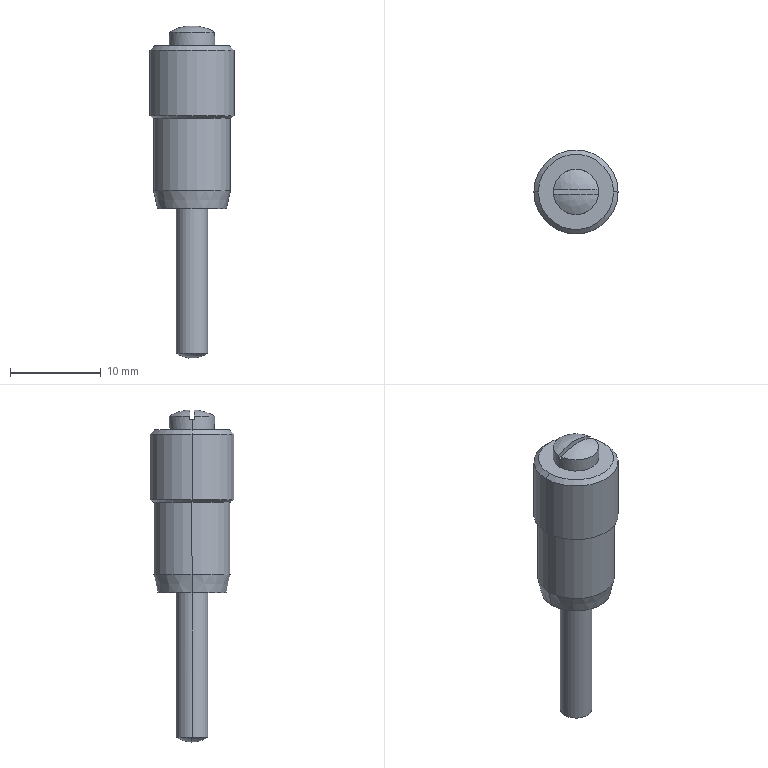Part | SolidWorks | features BaseBody 1 | 1 solid | 26 faces | box 9.3 x 9.3 x 36.697 mm | volume 794.178 mm3 | cylinder 10 | cone 6 | plane 6 | spline 4 | commonest cylinder face diameters 3.5 x2 5 x2 7 x2 8.5 x2 9.3 x2
STEP:
#1=CARTESIAN_POINT('',(-42.25,9.997,43.575));
#2=VERTEX_POINT('',#1);
#3=CARTESIAN_POINT('',(-45.75,9.997,43.575));
#4=VERTEX_POINT('',#3);
#5=CARTESIAN_POINT('',(-44.,9.997,43.575));
#6=DIRECTION('',(0.,0.,1.));
#7=DIRECTION('',(1.,0.,0.));
#8=AXIS2_PLACEMENT_3D('',#5,#6,#7);
#9=CIRCLE('',#8,1.75);
#10=EDGE_CURVE('',#2,#4,#9,.T.);
#11=ORIENTED_EDGE('',*,*,#10,.F.);
#12=CARTESIAN_POINT('',(-44.,9.997,46.011));
#13=DIRECTION('',(0.,1.,0.));
#14=DIRECTION('',(0.5924,0.,0.8057));
#15=AXIS2_PLACEMENT_3D('',#12,#13,#14);
#16=CIRCLE('',#15,3.);
#17=EDGE_CURVE('',#2,#4,#16,.T.);
#18=ORIENTED_EDGE('',*,*,#17,.T.);
#19=EDGE_LOOP('',(#11,#18));
#20=FACE_OUTER_BOUND('',#19,.T.);
#21=CARTESIAN_POINT('',(-42.232,9.997,43.588));
#22=CARTESIAN_POINT('',(-42.232,11.436,43.588));
#23=CARTESIAN_POINT('',(-42.972,12.543,44.132));
#24=CARTESIAN_POINT('',(-44.111,12.808,44.97));
#25=CARTESIAN_POINT('',(-43.324,9.997,42.791));
#26=CARTESIAN_POINT('',(-43.324,11.231,42.791));
#27=CARTESIAN_POINT('',(-43.959,12.18,43.258));
#28=CARTESIAN_POINT('',(-44.935,12.407,43.976));
#29=CARTESIAN_POINT('',(-44.676,9.997,42.791));
#30=CARTESIAN_POINT('',(-44.676,10.683,42.791));
#31=CARTESIAN_POINT('',(-45.029,11.21,43.05));
#32=CARTESIAN_POINT('',(-45.572,11.337,43.45));
#33=CARTESIAN_POINT('',(-45.768,9.997,43.588));
#34=CARTESIAN_POINT('',(-45.768,10.003,43.588));
#35=CARTESIAN_POINT('',(-45.771,10.007,43.59));
#36=CARTESIAN_POINT('',(-45.775,10.008,43.593));
#37=(BOUNDED_SURFACE()B_SPLINE_SURFACE(3,3,((#21,#22,#23,#24),(#25,#26,#27,#28),(#29,#30,#31,#32),(#33,#34,#35,#36)),.UNSPECIFIED.,.F.,.F.,.T.)B_SPLINE_SURFACE_WITH_KNOTS((4,4),(4,4),(0.,1.),(0.,1.),.UNSPECIFIED.)GEOMETRIC_REPRESENTATION_ITEM()RATIONAL_B_SPLINE_SURFACE(((1.,0.8464,0.8464,1.),(0.8719,0.738,0.738,0.8719),(0.8719,0.738,0.738,0.8719),(1.,0.8464,0.8464,1.)))REPRESENTATION_ITEM('')SURFACE());
#38=ADVANCED_FACE('',(#20),#37,.T.);
#39=CARTESIAN_POINT('',(-40.5,9.997,76.511));
#40=VERTEX_POINT('',#39);
#41=CARTESIAN_POINT('',(-47.5,9.997,76.511));
#42=VERTEX_POINT('',#41);
#43=CARTESIAN_POINT('',(-44.,9.997,76.511));
#44=DIRECTION('',(0.,0.,-1.));
#45=DIRECTION('',(-1.,0.,0.));
#46=AXIS2_PLACEMENT_3D('',#43,#44,#45);
#47=CIRCLE('',#46,3.5);
#48=EDGE_CURVE('',#40,#42,#47,.T.);
#49=ORIENTED_EDGE('',*,*,#48,.F.);
#50=CARTESIAN_POINT('',(-40.5,9.997,59.511));
#51=VERTEX_POINT('',#50);
#52=CARTESIAN_POINT('',(-40.5,9.997,76.511));
#53=DIRECTION('',(0.,0.,-1.));
#54=VECTOR('',#53,1000.);
#55=LINE('',#52,#54);
#56=EDGE_CURVE('',#40,#51,#55,.T.);
#57=ORIENTED_EDGE('',*,*,#56,.T.);
#58=CARTESIAN_POINT('',(-47.5,9.997,59.511));
#59=VERTEX_POINT('',#58);
#60=CARTESIAN_POINT('',(-44.,9.997,59.511));
#61=DIRECTION('',(0.,0.,1.));
#62=DIRECTION('',(-1.,0.,0.));
#63=AXIS2_PLACEMENT_3D('',#60,#61,#62);
#64=CIRCLE('',#63,3.5);
#65=EDGE_CURVE('',#59,#51,#64,.T.);
#66=ORIENTED_EDGE('',*,*,#65,.F.);
#67=CARTESIAN_POINT('',(-47.5,9.997,76.511));
#68=DIRECTION('',(0.,0.,-1.));
#69=VECTOR('',#68,1000.);
#70=LINE('',#67,#69);
#71=EDGE_CURVE('',#42,#59,#70,.T.);
#72=ORIENTED_EDGE('',*,*,#71,.F.);
#73=EDGE_LOOP('',(#49,#57,#66,#72));
#74=FACE_OUTER_BOUND('',#73,.T.);
#75=CARTESIAN_POINT('',(-44.,9.997,76.511));
#76=DIRECTION('',(0.,0.,-1.));
#77=DIRECTION('',(-1.,0.,0.));
#78=AXIS2_PLACEMENT_3D('',#75,#76,#77);
#79=CYLINDRICAL_SURFACE('',#78,3.5);
#80=ADVANCED_FACE('',(#74),#79,.F.);
#81=CARTESIAN_POINT('',(-47.8,9.997,59.511));
#82=VERTEX_POINT('',#81);
#83=CARTESIAN_POINT('',(-40.2,9.997,59.511));
#84=VERTEX_POINT('',#83);
#85=CARTESIAN_POINT('',(-44.,9.997,59.511));
#86=DIRECTION('',(0.,0.,-1.));
#87=DIRECTION('',(1.,0.,0.));
#88=AXIS2_PLACEMENT_3D('',#85,#86,#87);
#89=CIRCLE('',#88,3.8);
#90=EDGE_CURVE('',#82,#84,#89,.T.);
#91=ORIENTED_EDGE('',*,*,#90,.F.);
#92=CARTESIAN_POINT('',(-48.25,9.997,61.511));
#93=VERTEX_POINT('',#92);
#94=CARTESIAN_POINT('',(-48.25,9.997,61.511));
#95=DIRECTION('',(-0.2195,0.,0.9756));
#96=VECTOR('',#95,1000.);
#97=LINE('',#94,#96);
#98=EDGE_CURVE('',#82,#93,#97,.T.);
#99=ORIENTED_EDGE('',*,*,#98,.T.);
#100=CARTESIAN_POINT('',(-39.75,9.997,61.511));
#101=VERTEX_POINT('',#100);
#102=CARTESIAN_POINT('',(-44.,9.997,61.511));
#103=DIRECTION('',(0.,0.,-1.));
#104=DIRECTION('',(1.,0.,0.));
#105=AXIS2_PLACEMENT_3D('',#102,#103,#104);
#106=CIRCLE('',#105,4.25);
#107=EDGE_CURVE('',#93,#101,#106,.T.);
#108=ORIENTED_EDGE('',*,*,#107,.T.);
#109=CARTESIAN_POINT('',(-39.75,9.997,61.511));
#110=DIRECTION('',(0.2195,0.,0.9756));
#111=VECTOR('',#110,1000.);
#112=LINE('',#109,#111);
#113=EDGE_CURVE('',#84,#101,#112,.T.);
#114=ORIENTED_EDGE('',*,*,#113,.F.);
#115=EDGE_LOOP('',(#91,#99,#108,#114));
#116=FACE_OUTER_BOUND('',#115,.T.);
#117=CARTESIAN_POINT('',(-44.,9.997,61.511));
#118=DIRECTION('',(0.,0.,1.));
#119=DIRECTION('',(1.,0.,0.));
#120=AXIS2_PLACEMENT_3D('',#117,#118,#119);
#121=CONICAL_SURFACE('',#120,4.25,0.2213);
#122=ADVANCED_FACE('',(#116),#121,.T.);
#123=ORIENTED_EDGE('',*,*,#10,.T.);
#124=CARTESIAN_POINT('',(-45.75,9.997,76.511));
#125=VERTEX_POINT('',#124);
#126=CARTESIAN_POINT('',(-45.75,9.997,43.575));
#127=DIRECTION('',(0.,0.,1.));
#128=VECTOR('',#127,1000.);
#129=LINE('',#126,#128);
#130=EDGE_CURVE('',#4,#125,#129,.T.);
#131=ORIENTED_EDGE('',*,*,#130,.T.);
#132=CARTESIAN_POINT('',(-42.25,9.997,76.511));
#133=VERTEX_POINT('',#132);
#134=CARTESIAN_POINT('',(-44.,9.997,76.511));
#135=DIRECTION('',(0.,0.,1.));
#136=DIRECTION('',(1.,0.,0.));
#137=AXIS2_PLACEMENT_3D('',#134,#135,#136);
#138=CIRCLE('',#137,1.75);
#139=EDGE_CURVE('',#133,#125,#138,.T.);
#140=ORIENTED_EDGE('',*,*,#139,.F.);
#141=CARTESIAN_POINT('',(-42.25,9.997,43.575));
#142=DIRECTION('',(0.,0.,1.));
#143=VECTOR('',#142,1000.);
#144=LINE('',#141,#143);
#145=EDGE_CURVE('',#2,#133,#144,.T.);
#146=ORIENTED_EDGE('',*,*,#145,.F.);
#147=EDGE_LOOP('',(#123,#131,#140,#146));
#148=FACE_OUTER_BOUND('',#147,.T.);
#149=CARTESIAN_POINT('',(-44.,9.997,43.575));
#150=DIRECTION('',(0.,0.,1.));
#151=DIRECTION('',(1.,0.,0.));
#152=AXIS2_PLACEMENT_3D('',#149,#150,#151);
#153=CYLINDRICAL_SURFACE('',#152,1.75);
#154=ADVANCED_FACE('',(#148),#153,.T.);
#155=ORIENTED_EDGE('',*,*,#107,.F.);
#156=CARTESIAN_POINT('',(-48.25,9.997,69.511));
#157=VERTEX_POINT('',#156);
#158=CARTESIAN_POINT('',(-48.25,9.997,61.511));
#159=DIRECTION('',(0.,0.,1.));
#160=VECTOR('',#159,1000.);
#161=LINE('',#158,#160);
#162=EDGE_CURVE('',#93,#157,#161,.T.);
#163=ORIENTED_EDGE('',*,*,#162,.T.);
#164=CARTESIAN_POINT('',(-39.75,9.997,69.511));
#165=VERTEX_POINT('',#164);
#166=CARTESIAN_POINT('',(-44.,9.997,69.511));
#167=DIRECTION('',(0.,0.,-1.));
#168=DIRECTION('',(1.,0.,0.));
#169=AXIS2_PLACEMENT_3D('',#166,#167,#168);
#170=CIRCLE('',#169,4.25);
#171=EDGE_CURVE('',#157,#165,#170,.T.);
#172=ORIENTED_EDGE('',*,*,#171,.T.);
#173=CARTESIAN_POINT('',(-39.75,9.997,61.511));
#174=DIRECTION('',(0.,0.,1.));
#175=VECTOR('',#174,1000.);
#176=LINE('',#173,#175);
#177=EDGE_CURVE('',#101,#165,#176,.T.);
#178=ORIENTED_EDGE('',*,*,#177,.F.);
#179=EDGE_LOOP('',(#155,#163,#172,#178));
#180=FACE_OUTER_BOUND('',#179,.T.);
#181=CARTESIAN_POINT('',(-44.,9.997,61.511));
#182=DIRECTION('',(0.,0.,1.));
#183=DIRECTION('',(1.,0.,0.));
#184=AXIS2_PLACEMENT_3D('',#181,#182,#183);
#185=CYLINDRICAL_SURFACE('',#184,4.25);
#186=ADVANCED_FACE('',(#180),#185,.T.);
#187=ORIENTED_EDGE('',*,*,#171,.F.);
#188=CARTESIAN_POINT('',(-48.65,9.997,69.761));
#189=VERTEX_POINT('',#188);
#190=CARTESIAN_POINT('',(-48.65,9.997,69.761));
#191=DIRECTION('',(-0.848,0.,0.53));
#192=VECTOR('',#191,1000.);
#193=LINE('',#190,#192);
#194=EDGE_CURVE('',#157,#189,#193,.T.);
#195=ORIENTED_EDGE('',*,*,#194,.T.);
#196=CARTESIAN_POINT('',(-39.35,9.997,69.761));
#197=VERTEX_POINT('',#196);
#198=CARTESIAN_POINT('',(-44.,9.997,69.761));
#199=DIRECTION('',(0.,0.,-1.));
#200=DIRECTION('',(1.,0.,0.));
#201=AXIS2_PLACEMENT_3D('',#198,#199,#200);
#202=CIRCLE('',#201,4.65);
#203=EDGE_CURVE('',#189,#197,#202,.T.);
#204=ORIENTED_EDGE('',*,*,#203,.T.);
#205=CARTESIAN_POINT('',(-39.35,9.997,69.761));
#206=DIRECTION('',(0.848,0.,0.53));
#207=VECTOR('',#206,1000.);
#208=LINE('',#205,#207);
#209=EDGE_CURVE('',#165,#197,#208,.T.);
#210=ORIENTED_EDGE('',*,*,#209,.F.);
#211=EDGE_LOOP('',(#187,#195,#204,#210));
#212=FACE_OUTER_BOUND('',#211,.T.);
#213=CARTESIAN_POINT('',(-44.,9.997,69.761));
#214=DIRECTION('',(0.,0.,1.));
#215=DIRECTION('',(1.,0.,0.));
#216=AXIS2_PLACEMENT_3D('',#213,#214,#215);
#217=CONICAL_SURFACE('',#216,4.65,1.012);
#218=ADVANCED_FACE('',(#212),#217,.T.);
#219=ORIENTED_EDGE('',*,*,#203,.F.);
#220=CARTESIAN_POINT('',(-48.65,9.997,77.011));
#221=VERTEX_POINT('',#220);
#222=CARTESIAN_POINT('',(-48.65,9.997,69.761));
#223=DIRECTION('',(0.,0.,1.));
#224=VECTOR('',#223,1000.);
#225=LINE('',#222,#224);
#226=EDGE_CURVE('',#189,#221,#225,.T.);
#227=ORIENTED_EDGE('',*,*,#226,.T.);
#228=CARTESIAN_POINT('',(-39.35,9.997,77.011));
#229=VERTEX_POINT('',#228);
#230=CARTESIAN_POINT('',(-44.,9.997,77.011));
#231=DIRECTION('',(0.,0.,-1.));
#232=DIRECTION('',(1.,0.,0.));
#233=AXIS2_PLACEMENT_3D('',#230,#231,#232);
#234=CIRCLE('',#233,4.65);
#235=EDGE_CURVE('',#221,#229,#234,.T.);
#236=ORIENTED_EDGE('',*,*,#235,.T.);
#237=CARTESIAN_POINT('',(-39.35,9.997,69.761));
#238=DIRECTION('',(0.,0.,1.));
#239=VECTOR('',#238,1000.);
#240=LINE('',#237,#239);
#241=EDGE_CURVE('',#197,#229,#240,.T.);
#242=ORIENTED_EDGE('',*,*,#241,.F.);
#243=EDGE_LOOP('',(#219,#227,#236,#242));
#244=FACE_OUTER_BOUND('',#243,.T.);
#245=CARTESIAN_POINT('',(-44.,9.997,69.761));
#246=DIRECTION('',(0.,0.,1.));
#247=DIRECTION('',(1.,0.,0.));
#248=AXIS2_PLACEMENT_3D('',#245,#246,#247);
#249=CYLINDRICAL_SURFACE('',#248,4.65);
#250=ADVANCED_FACE('',(#244),#249,.T.);
#251=CARTESIAN_POINT('',(-48.15,9.997,77.511));
#252=VERTEX_POINT('',#251);
#253=CARTESIAN_POINT('',(-39.85,9.997,77.511));
#254=VERTEX_POINT('',#253);
#255=CARTESIAN_POINT('',(-44.,9.997,77.511));
#256=DIRECTION('',(0.,0.,-1.));
#257=DIRECTION('',(-1.,0.,0.));
#258=AXIS2_PLACEMENT_3D('',#255,#256,#257);
#259=CIRCLE('',#258,4.15);
#260=EDGE_CURVE('',#252,#254,#259,.T.);
#261=ORIENTED_EDGE('',*,*,#260,.T.);
#262=CARTESIAN_POINT('',(-39.35,9.997,77.011));
#263=DIRECTION('',(0.7071,0.,-0.7071));
#264=VECTOR('',#263,1000.);
#265=LINE('',#262,#264);
#266=EDGE_CURVE('',#254,#229,#265,.T.);
#267=ORIENTED_EDGE('',*,*,#266,.T.);
#268=ORIENTED_EDGE('',*,*,#235,.F.);
#269=CARTESIAN_POINT('',(-48.65,9.997,77.011));
#270=DIRECTION('',(-0.7071,0.,-0.7071));
#271=VECTOR('',#270,1000.);
#272=LINE('',#269,#271);
#273=EDGE_CURVE('',#252,#221,#272,.T.);
#274=ORIENTED_EDGE('',*,*,#273,.F.);
#275=EDGE_LOOP('',(#261,#267,#268,#274));
#276=FACE_OUTER_BOUND('',#275,.T.);
#277=CARTESIAN_POINT('',(-44.,9.997,77.011));
#278=DIRECTION('',(0.,0.,-1.));
#279=DIRECTION('',(-1.,0.,0.));
#280=AXIS2_PLACEMENT_3D('',#277,#278,#279);
#281=CONICAL_SURFACE('',#280,4.65,0.7854);
#282=ADVANCED_FACE('',(#276),#281,.T.);
#283=CARTESIAN_POINT('',(-41.5,9.997,78.661));
#284=VERTEX_POINT('',#283);
#285=CARTESIAN_POINT('',(-41.513,10.247,78.661));
#286=VERTEX_POINT('',#285);
#287=CARTESIAN_POINT('',(-44.,9.997,78.661));
#288=DIRECTION('',(0.,0.,1.));
#289=DIRECTION('',(-1.,0.,0.));
#290=AXIS2_PLACEMENT_3D('',#287,#288,#289);
#291=CIRCLE('',#290,2.5);
#292=EDGE_CURVE('',#284,#286,#291,.T.);
#293=ORIENTED_EDGE('',*,*,#292,.F.);
#294=CARTESIAN_POINT('',(-41.5,9.997,77.511));
#295=VERTEX_POINT('',#294);
#296=CARTESIAN_POINT('',(-41.5,9.997,79.011));
#297=DIRECTION('',(0.,0.,-1.));
#298=VECTOR('',#297,1000.);
#299=LINE('',#296,#298);
#300=EDGE_CURVE('',#284,#295,#299,.T.);
#301=ORIENTED_EDGE('',*,*,#300,.T.);
#302=CARTESIAN_POINT('',(-46.5,9.997,77.511));
#303=VERTEX_POINT('',#302);
#304=CARTESIAN_POINT('',(-44.,9.997,77.511));
#305=DIRECTION('',(0.,0.,-1.));
#306=DIRECTION('',(-1.,0.,0.));
#307=AXIS2_PLACEMENT_3D('',#304,#305,#306);
#308=CIRCLE('',#307,2.5);
#309=EDGE_CURVE('',#303,#295,#308,.T.);
#310=ORIENTED_EDGE('',*,*,#309,.F.);
#311=CARTESIAN_POINT('',(-46.5,9.997,78.661));
#312=VERTEX_POINT('',#311);
#313=CARTESIAN_POINT('',(-46.5,9.997,79.011));
#314=DIRECTION('',(0.,0.,-1.));
#315=VECTOR('',#314,1000.);
#316=LINE('',#313,#315);
#317=EDGE_CURVE('',#312,#303,#316,.T.);
#318=ORIENTED_EDGE('',*,*,#317,.F.);
#319=CARTESIAN_POINT('',(-46.487,10.247,78.661));
#320=VERTEX_POINT('',#319);
#321=CARTESIAN_POINT('',(-44.,9.997,78.661));
#322=DIRECTION('',(0.,0.,1.));
#323=DIRECTION('',(-1.,0.,0.));
#324=AXIS2_PLACEMENT_3D('',#321,#322,#323);
#325=CIRCLE('',#324,2.5);
#326=EDGE_CURVE('',#320,#312,#325,.T.);
#327=ORIENTED_EDGE('',*,*,#326,.F.);
#328=CARTESIAN_POINT('',(-46.487,10.247,79.011));
#329=VERTEX_POINT('',#328);
#330=CARTESIAN_POINT('',(-46.487,10.247,78.661));
#331=DIRECTION('',(0.,0.,1.));
#332=VECTOR('',#331,1000.);
#333=LINE('',#330,#332);
#334=EDGE_CURVE('',#320,#329,#333,.T.);
#335=ORIENTED_EDGE('',*,*,#334,.T.);
#336=CARTESIAN_POINT('',(-41.513,10.247,79.011));
#337=VERTEX_POINT('',#336);
#338=CARTESIAN_POINT('',(-44.,9.997,79.011));
#339=DIRECTION('',(0.,0.,-1.));
#340=DIRECTION('',(-1.,0.,0.));
#341=AXIS2_PLACEMENT_3D('',#338,#339,#340);
#342=CIRCLE('',#341,2.5);
#343=EDGE_CURVE('',#329,#337,#342,.T.);
#344=ORIENTED_EDGE('',*,*,#343,.T.);
#345=CARTESIAN_POINT('',(-41.513,10.247,78.661));
#346=DIRECTION('',(0.,0.,-1.));
#347=VECTOR('',#346,1000.);
#348=LINE('',#345,#347);
#349=EDGE_CURVE('',#337,#286,#348,.T.);
#350=ORIENTED_EDGE('',*,*,#349,.T.);
#351=EDGE_LOOP('',(#293,#301,#310,#318,#327,#335,#344,#350));
#352=FACE_OUTER_BOUND('',#351,.T.);
#353=CARTESIAN_POINT('',(-44.,9.997,79.011));
#354=DIRECTION('',(0.,0.,-1.));
#355=DIRECTION('',(-1.,0.,0.));
#356=AXIS2_PLACEMENT_3D('',#353,#354,#355);
#357=CYLINDRICAL_SURFACE('',#356,2.5);
#358=ADVANCED_FACE('',(#352),#357,.T.);
#359=ORIENTED_EDGE('',*,*,#56,.F.);
#360=CARTESIAN_POINT('',(-44.,9.997,76.511));
#361=DIRECTION('',(0.,0.,-1.));
#362=DIRECTION('',(-1.,0.,0.));
#363=AXIS2_PLACEMENT_3D('',#360,#361,#362);
#364=CIRCLE('',#363,3.5);
#365=EDGE_CURVE('',#42,#40,#364,.T.);
#366=ORIENTED_EDGE('',*,*,#365,.F.);
#367=ORIENTED_EDGE('',*,*,#71,.T.);
#368=CARTESIAN_POINT('',(-44.,9.997,59.511));
#369=DIRECTION('',(0.,0.,1.));
#370=DIRECTION('',(-1.,0.,0.));
#371=AXIS2_PLACEMENT_3D('',#368,#369,#370);
#372=CIRCLE('',#371,3.5);
#373=EDGE_CURVE('',#51,#59,#372,.T.);
#374=ORIENTED_EDGE('',*,*,#373,.F.);
#375=EDGE_LOOP('',(#359,#366,#367,#374));
#376=FACE_OUTER_BOUND('',#375,.T.);
#377=CARTESIAN_POINT('',(-44.,9.997,76.511));
#378=DIRECTION('',(0.,0.,-1.));
#379=DIRECTION('',(-1.,0.,0.));
#380=AXIS2_PLACEMENT_3D('',#377,#378,#379);
#381=CYLINDRICAL_SURFACE('',#380,3.5);
#382=ADVANCED_FACE('',(#376),#381,.F.);
#383=ORIENTED_EDGE('',*,*,#65,.T.);
#384=ORIENTED_EDGE('',*,*,#373,.T.);
#385=EDGE_LOOP('',(#383,#384));
#386=FACE_BOUND('',#385,.T.);
#387=CARTESIAN_POINT('',(-44.,9.997,59.511));
#388=DIRECTION('',(0.,0.,-1.));
#389=DIRECTION('',(1.,0.,0.));
#390=AXIS2_PLACEMENT_3D('',#387,#388,#389);
#391=CIRCLE('',#390,3.8);
#392=EDGE_CURVE('',#84,#82,#391,.T.);
#393=ORIENTED_EDGE('',*,*,#392,.T.);
#394=ORIENTED_EDGE('',*,*,#90,.T.);
#395=EDGE_LOOP('',(#393,#394));
#396=FACE_OUTER_BOUND('',#395,.T.);
#397=CARTESIAN_POINT('',(-47.8,6.197,59.511));
#398=DIRECTION('',(0.,0.,-1.));
#399=DIRECTION('',(-1.,0.,0.));
#400=AXIS2_PLACEMENT_3D('',#397,#398,#399);
#401=PLANE('',#400);
#402=ADVANCED_FACE('',(#386,#396),#401,.T.);
#403=ORIENTED_EDGE('',*,*,#139,.T.);
#404=CARTESIAN_POINT('',(-44.,9.997,76.511));
#405=DIRECTION('',(0.,0.,1.));
#406=DIRECTION('',(1.,0.,0.));
#407=AXIS2_PLACEMENT_3D('',#404,#405,#406);
#408=CIRCLE('',#407,1.75);
#409=EDGE_CURVE('',#125,#133,#408,.T.);
#410=ORIENTED_EDGE('',*,*,#409,.T.);
#411=EDGE_LOOP('',(#403,#410));
#412=FACE_BOUND('',#411,.T.);
#413=ORIENTED_EDGE('',*,*,#365,.T.);
#414=ORIENTED_EDGE('',*,*,#48,.T.);
#415=EDGE_LOOP('',(#413,#414));
#416=FACE_OUTER_BOUND('',#415,.T.);
#417=CARTESIAN_POINT('',(-47.5,6.497,76.511));
#418=DIRECTION('',(0.,0.,-1.));
#419=DIRECTION('',(-1.,0.,0.));
#420=AXIS2_PLACEMENT_3D('',#417,#418,#419);
#421=PLANE('',#420);
#422=ADVANCED_FACE('',(#412,#416),#421,.T.);
#423=ORIENTED_EDGE('',*,*,#98,.F.);
#424=ORIENTED_EDGE('',*,*,#392,.F.);
#425=ORIENTED_EDGE('',*,*,#113,.T.);
#426=CARTESIAN_POINT('',(-44.,9.997,61.511));
#427=DIRECTION('',(0.,0.,-1.));
#428=DIRECTION('',(1.,0.,0.));
#429=AXIS2_PLACEMENT_3D('',#426,#427,#428);
#430=CIRCLE('',#429,4.25);
#431=EDGE_CURVE('',#101,#93,#430,.T.);
#432=ORIENTED_EDGE('',*,*,#431,.T.);
#433=EDGE_LOOP('',(#423,#424,#425,#432));
#434=FACE_OUTER_BOUND('',#433,.T.);
#435=CARTESIAN_POINT('',(-44.,9.997,61.511));
#436=DIRECTION('',(0.,0.,1.));
#437=DIRECTION('',(1.,0.,0.));
#438=AXIS2_PLACEMENT_3D('',#435,#436,#437);
#439=CONICAL_SURFACE('',#438,4.25,0.2213);
#440=ADVANCED_FACE('',(#434),#439,.T.);
#441=ORIENTED_EDGE('',*,*,#130,.F.);
#442=CARTESIAN_POINT('',(-44.,9.997,43.575));
#443=DIRECTION('',(0.,0.,1.));
#444=DIRECTION('',(1.,0.,0.));
#445=AXIS2_PLACEMENT_3D('',#442,#443,#444);
#446=CIRCLE('',#445,1.75);
#447=EDGE_CURVE('',#4,#2,#446,.T.);
#448=ORIENTED_EDGE('',*,*,#447,.T.);
#449=ORIENTED_EDGE('',*,*,#145,.T.);
#450=ORIENTED_EDGE('',*,*,#409,.F.);
#451=EDGE_LOOP('',(#441,#448,#449,#450));
#452=FACE_OUTER_BOUND('',#451,.T.);
#453=CARTESIAN_POINT('',(-44.,9.997,43.575));
#454=DIRECTION('',(0.,0.,1.));
#455=DIRECTION('',(1.,0.,0.));
#456=AXIS2_PLACEMENT_3D('',#453,#454,#455);
#457=CYLINDRICAL_SURFACE('',#456,1.75);
#458=ADVANCED_FACE('',(#452),#457,.T.);
#459=ORIENTED_EDGE('',*,*,#162,.F.);
#460=ORIENTED_EDGE('',*,*,#431,.F.);
#461=ORIENTED_EDGE('',*,*,#177,.T.);
#462=CARTESIAN_POINT('',(-44.,9.997,69.511));
#463=DIRECTION('',(0.,0.,-1.));
#464=DIRECTION('',(1.,0.,0.));
#465=AXIS2_PLACEMENT_3D('',#462,#463,#464);
#466=CIRCLE('',#465,4.25);
#467=EDGE_CURVE('',#165,#157,#466,.T.);
#468=ORIENTED_EDGE('',*,*,#467,.T.);
#469=EDGE_LOOP('',(#459,#460,#461,#468));
#470=FACE_OUTER_BOUND('',#469,.T.);
#471=CARTESIAN_POINT('',(-44.,9.997,61.511));
#472=DIRECTION('',(0.,0.,1.));
#473=DIRECTION('',(1.,0.,0.));
#474=AXIS2_PLACEMENT_3D('',#471,#472,#473);
#475=CYLINDRICAL_SURFACE('',#474,4.25);
#476=ADVANCED_FACE('',(#470),#475,.T.);
#477=ORIENTED_EDGE('',*,*,#17,.F.);
#478=ORIENTED_EDGE('',*,*,#447,.F.);
#479=EDGE_LOOP('',(#477,#478));
#480=FACE_OUTER_BOUND('',#479,.T.);
#481=CARTESIAN_POINT('',(-44.153,7.177,45.));
#482=CARTESIAN_POINT('',(-42.992,7.42,44.147));
#483=CARTESIAN_POINT('',(-42.232,8.536,43.588));
#484=CARTESIAN_POINT('',(-42.232,9.997,43.588));
#485=CARTESIAN_POINT('',(-44.971,7.579,44.002));
#486=CARTESIAN_POINT('',(-43.976,7.787,43.27));
#487=CARTESIAN_POINT('',(-43.324,8.744,42.791));
#488=CARTESIAN_POINT('',(-43.324,9.997,42.791));
#489=CARTESIAN_POINT('',(-45.591,8.653,43.464));
#490=CARTESIAN_POINT('',(-45.038,8.769,43.057));
#491=CARTESIAN_POINT('',(-44.676,9.301,42.791));
#492=CARTESIAN_POINT('',(-44.676,9.997,42.791));
#493=CARTESIAN_POINT('',(-45.776,9.986,43.593));
#494=CARTESIAN_POINT('',(-45.771,9.987,43.59));
#495=CARTESIAN_POINT('',(-45.768,9.991,43.588));
#496=CARTESIAN_POINT('',(-45.768,9.997,43.588));
#497=(BOUNDED_SURFACE()B_SPLINE_SURFACE(3,3,((#481,#482,#483,#484),(#485,#486,#487,#488),(#489,#490,#491,#492),(#493,#494,#495,#496)),.UNSPECIFIED.,.F.,.F.,.F.)B_SPLINE_SURFACE_WITH_KNOTS((4,4),(4,4),(0.,1.),(0.,1.),.UNSPECIFIED.)GEOMETRIC_REPRESENTATION_ITEM()RATIONAL_B_SPLINE_SURFACE(((1.,0.8425,0.8425,1.),(0.8719,0.7345,0.7345,0.8719),(0.8719,0.7345,0.7345,0.8719),(1.,0.8425,0.8425,1.)))REPRESENTATION_ITEM('')SURFACE());
#498=ADVANCED_FACE('',(#480),#497,.T.);
#499=ORIENTED_EDGE('',*,*,#194,.F.);
#500=ORIENTED_EDGE('',*,*,#467,.F.);
#501=ORIENTED_EDGE('',*,*,#209,.T.);
#502=CARTESIAN_POINT('',(-44.,9.997,69.761));
#503=DIRECTION('',(0.,0.,-1.));
#504=DIRECTION('',(1.,0.,0.));
#505=AXIS2_PLACEMENT_3D('',#502,#503,#504);
#506=CIRCLE('',#505,4.65);
#507=EDGE_CURVE('',#197,#189,#506,.T.);
#508=ORIENTED_EDGE('',*,*,#507,.T.);
#509=EDGE_LOOP('',(#499,#500,#501,#508));
#510=FACE_OUTER_BOUND('',#509,.T.);
#511=CARTESIAN_POINT('',(-44.,9.997,69.761));
#512=DIRECTION('',(0.,0.,1.));
#513=DIRECTION('',(1.,0.,0.));
#514=AXIS2_PLACEMENT_3D('',#511,#512,#513);
#515=CONICAL_SURFACE('',#514,4.65,1.012);
#516=ADVANCED_FACE('',(#510),#515,.T.);
#517=ORIENTED_EDGE('',*,*,#226,.F.);
#518=ORIENTED_EDGE('',*,*,#507,.F.);
#519=ORIENTED_EDGE('',*,*,#241,.T.);
#520=CARTESIAN_POINT('',(-44.,9.997,77.011));
#521=DIRECTION('',(0.,0.,-1.));
#522=DIRECTION('',(1.,0.,0.));
#523=AXIS2_PLACEMENT_3D('',#520,#521,#522);
#524=CIRCLE('',#523,4.65);
#525=EDGE_CURVE('',#229,#221,#524,.T.);
#526=ORIENTED_EDGE('',*,*,#525,.T.);
#527=EDGE_LOOP('',(#517,#518,#519,#526));
#528=FACE_OUTER_BOUND('',#527,.T.);
#529=CARTESIAN_POINT('',(-44.,9.997,69.761));
#530=DIRECTION('',(0.,0.,1.));
#531=DIRECTION('',(1.,0.,0.));
#532=AXIS2_PLACEMENT_3D('',#529,#530,#531);
#533=CYLINDRICAL_SURFACE('',#532,4.65);
#534=ADVANCED_FACE('',(#528),#533,.T.);
#535=ORIENTED_EDGE('',*,*,#266,.F.);
#536=CARTESIAN_POINT('',(-44.,9.997,77.511));
#537=DIRECTION('',(0.,0.,-1.));
#538=DIRECTION('',(-1.,0.,0.));
#539=AXIS2_PLACEMENT_3D('',#536,#537,#538);
#540=CIRCLE('',#539,4.15);
#541=EDGE_CURVE('',#254,#252,#540,.T.);
#542=ORIENTED_EDGE('',*,*,#541,.T.);
#543=ORIENTED_EDGE('',*,*,#273,.T.);
#544=ORIENTED_EDGE('',*,*,#525,.F.);
#545=EDGE_LOOP('',(#535,#542,#543,#544));
#546=FACE_OUTER_BOUND('',#545,.T.);
#547=CARTESIAN_POINT('',(-44.,9.997,77.011));
#548=DIRECTION('',(0.,0.,-1.));
#549=DIRECTION('',(-1.,0.,0.));
#550=AXIS2_PLACEMENT_3D('',#547,#548,#549);
#551=CONICAL_SURFACE('',#550,4.65,0.7854);
#552=ADVANCED_FACE('',(#546),#551,.T.);
#553=ORIENTED_EDGE('',*,*,#309,.T.);
#554=CARTESIAN_POINT('',(-44.,9.997,77.511));
#555=DIRECTION('',(0.,0.,-1.));
#556=DIRECTION('',(-1.,0.,0.));
#557=AXIS2_PLACEMENT_3D('',#554,#555,#556);
#558=CIRCLE('',#557,2.5);
#559=EDGE_CURVE('',#295,#303,#558,.T.);
#560=ORIENTED_EDGE('',*,*,#559,.T.);
#561=EDGE_LOOP('',(#553,#560));
#562=FACE_BOUND('',#561,.T.);
#563=ORIENTED_EDGE('',*,*,#260,.F.);
#564=ORIENTED_EDGE('',*,*,#541,.F.);
#565=EDGE_LOOP('',(#563,#564));
#566=FACE_OUTER_BOUND('',#565,.T.);
#567=CARTESIAN_POINT('',(-48.15,14.147,77.511));
#568=DIRECTION('',(0.,0.,1.));
#569=DIRECTION('',(1.,0.,0.));
#570=AXIS2_PLACEMENT_3D('',#567,#568,#569);
#571=PLANE('',#570);
#572=ADVANCED_FACE('',(#562,#566),#571,.T.);
#573=ORIENTED_EDGE('',*,*,#300,.F.);
#574=CARTESIAN_POINT('',(-41.513,9.747,78.661));
#575=VERTEX_POINT('',#574);
#576=CARTESIAN_POINT('',(-44.,9.997,78.661));
#577=DIRECTION('',(0.,0.,1.));
#578=DIRECTION('',(-1.,0.,0.));
#579=AXIS2_PLACEMENT_3D('',#576,#577,#578);
#580=CIRCLE('',#579,2.5);
#581=EDGE_CURVE('',#575,#284,#580,.T.);
#582=ORIENTED_EDGE('',*,*,#581,.F.);
#583=CARTESIAN_POINT('',(-41.513,9.747,79.011));
#584=VERTEX_POINT('',#583);
#585=CARTESIAN_POINT('',(-41.513,9.747,79.709));
#586=DIRECTION('',(0.,0.,1.));
#587=VECTOR('',#586,1000.);
#588=LINE('',#585,#587);
#589=EDGE_CURVE('',#575,#584,#588,.T.);
#590=ORIENTED_EDGE('',*,*,#589,.T.);
#591=CARTESIAN_POINT('',(-46.487,9.747,79.011));
#592=VERTEX_POINT('',#591);
#593=CARTESIAN_POINT('',(-44.,9.997,79.011));
#594=DIRECTION('',(0.,0.,-1.));
#595=DIRECTION('',(-1.,0.,0.));
#596=AXIS2_PLACEMENT_3D('',#593,#594,#595);
#597=CIRCLE('',#596,2.5);
#598=EDGE_CURVE('',#584,#592,#597,.T.);
#599=ORIENTED_EDGE('',*,*,#598,.T.);
#600=CARTESIAN_POINT('',(-46.487,9.747,78.661));
#601=VERTEX_POINT('',#600);
#602=CARTESIAN_POINT('',(-46.487,9.747,79.709));
#603=DIRECTION('',(0.,0.,-1.));
#604=VECTOR('',#603,1000.);
#605=LINE('',#602,#604);
#606=EDGE_CURVE('',#592,#601,#605,.T.);
#607=ORIENTED_EDGE('',*,*,#606,.T.);
#608=CARTESIAN_POINT('',(-44.,9.997,78.661));
#609=DIRECTION('',(0.,0.,1.));
#610=DIRECTION('',(-1.,0.,0.));
#611=AXIS2_PLACEMENT_3D('',#608,#609,#610);
#612=CIRCLE('',#611,2.5);
#613=EDGE_CURVE('',#312,#601,#612,.T.);
#614=ORIENTED_EDGE('',*,*,#613,.F.);
#615=ORIENTED_EDGE('',*,*,#317,.T.);
#616=ORIENTED_EDGE('',*,*,#559,.F.);
#617=EDGE_LOOP('',(#573,#582,#590,#599,#607,#614,#615,#616));
#618=FACE_OUTER_BOUND('',#617,.T.);
#619=CARTESIAN_POINT('',(-44.,9.997,79.011));
#620=DIRECTION('',(0.,0.,-1.));
#621=DIRECTION('',(-1.,0.,0.));
#622=AXIS2_PLACEMENT_3D('',#619,#620,#621);
#623=CYLINDRICAL_SURFACE('',#622,2.5);
#624=ADVANCED_FACE('',(#618),#623,.T.);
#625=CARTESIAN_POINT('',(-46.487,10.247,79.011));
#626=CARTESIAN_POINT('',(-46.112,10.247,79.24));
#627=CARTESIAN_POINT('',(-45.714,10.247,79.413));
#628=CARTESIAN_POINT('',(-45.084,10.247,79.589));
#629=CARTESIAN_POINT('',(-44.868,10.247,79.635));
#630=CARTESIAN_POINT('',(-44.436,10.247,79.694));
#631=CARTESIAN_POINT('',(-44.22,10.247,79.709));
#632=CARTESIAN_POINT('',(-43.569,10.247,79.709));
#633=CARTESIAN_POINT('',(-43.128,10.247,79.649));
#634=CARTESIAN_POINT('',(-42.501,10.247,79.473));
#635=CARTESIAN_POINT('',(-42.297,10.247,79.401));
#636=CARTESIAN_POINT('',(-41.897,10.247,79.227));
#637=CARTESIAN_POINT('',(-41.7,10.247,79.126));
#638=CARTESIAN_POINT('',(-41.513,10.247,79.011));
#639=B_SPLINE_CURVE_WITH_KNOTS('',3,(#625,#626,#627,#628,#629,#630,#631,#632,#633,#634,#635,#636,#637,#638),.UNSPECIFIED.,.F.,.F.,(4,2,2,2,2,2,4),(0.,0.001301,0.001951,0.002602,0.003903,0.004553,0.005203),.UNSPECIFIED.);
#640=EDGE_CURVE('',#329,#337,#639,.T.);
#641=ORIENTED_EDGE('',*,*,#640,.T.);
#642=ORIENTED_EDGE('',*,*,#343,.F.);
#643=EDGE_LOOP('',(#641,#642));
#644=FACE_OUTER_BOUND('',#643,.T.);
#645=CARTESIAN_POINT('',(-41.503,10.218,79.007));
#646=CARTESIAN_POINT('',(-41.608,10.206,79.072));
#647=CARTESIAN_POINT('',(-41.677,10.113,79.115));
#648=CARTESIAN_POINT('',(-41.674,9.99,79.113));
#649=CARTESIAN_POINT('',(-41.694,11.986,79.028));
#650=CARTESIAN_POINT('',(-42.633,11.878,79.608));
#651=CARTESIAN_POINT('',(-43.257,11.045,79.993));
#652=CARTESIAN_POINT('',(-43.228,9.936,79.976));
#653=CARTESIAN_POINT('',(-42.327,13.47,78.28));
#654=CARTESIAN_POINT('',(-43.967,13.281,79.293));
#655=CARTESIAN_POINT('',(-45.055,11.827,79.965));
#656=CARTESIAN_POINT('',(-45.005,9.891,79.934));
#657=CARTESIAN_POINT('',(-43.229,14.262,76.967));
#658=CARTESIAN_POINT('',(-45.243,14.03,78.211));
#659=CARTESIAN_POINT('',(-46.579,12.244,79.036));
#660=CARTESIAN_POINT('',(-46.518,9.867,78.998));
#661=(BOUNDED_SURFACE()B_SPLINE_SURFACE(3,3,((#645,#646,#647,#648),(#649,#650,#651,#652),(#653,#654,#655,#656),(#657,#658,#659,#660)),.UNSPECIFIED.,.F.,.F.,.F.)B_SPLINE_SURFACE_WITH_KNOTS((4,4),(4,4),(0.,1.),(0.,1.),.UNSPECIFIED.)GEOMETRIC_REPRESENTATION_ITEM()RATIONAL_B_SPLINE_SURFACE(((1.,0.8203,0.8203,1.),(0.9084,0.7452,0.7452,0.9084),(0.9084,0.7452,0.7452,0.9084),(1.,0.8203,0.8203,1.)))REPRESENTATION_ITEM('')SURFACE());
#662=ADVANCED_FACE('',(#644),#661,.T.);
#663=CARTESIAN_POINT('',(-41.513,9.747,79.011));
#664=CARTESIAN_POINT('',(-41.888,9.747,79.24));
#665=CARTESIAN_POINT('',(-42.294,9.747,79.415));
#666=CARTESIAN_POINT('',(-42.92,9.747,79.59));
#667=CARTESIAN_POINT('',(-43.132,9.747,79.635));
#668=CARTESIAN_POINT('',(-43.566,9.747,79.694));
#669=CARTESIAN_POINT('',(-43.785,9.747,79.709));
#670=CARTESIAN_POINT('',(-44.22,9.747,79.709));
#671=CARTESIAN_POINT('',(-44.436,9.747,79.694));
#672=CARTESIAN_POINT('',(-44.866,9.747,79.635));
#673=CARTESIAN_POINT('',(-45.082,9.747,79.59));
#674=CARTESIAN_POINT('',(-45.713,9.747,79.413));
#675=CARTESIAN_POINT('',(-46.112,9.747,79.24));
#676=CARTESIAN_POINT('',(-46.487,9.747,79.011));
#677=B_SPLINE_CURVE_WITH_KNOTS('',3,(#663,#664,#665,#666,#667,#668,#669,#670,#671,#672,#673,#674,#675,#676),.UNSPECIFIED.,.F.,.F.,(4,2,2,2,2,2,4),(0.,0.001317,0.001976,0.002634,0.003293,0.003951,0.005268),.UNSPECIFIED.);
#678=EDGE_CURVE('',#584,#592,#677,.T.);
#679=ORIENTED_EDGE('',*,*,#678,.T.);
#680=ORIENTED_EDGE('',*,*,#598,.F.);
#681=EDGE_LOOP('',(#679,#680));
#682=FACE_OUTER_BOUND('',#681,.T.);
#683=CARTESIAN_POINT('',(-43.108,5.721,76.892));
#684=CARTESIAN_POINT('',(-45.055,5.868,78.095));
#685=CARTESIAN_POINT('',(-46.423,7.504,78.94));
#686=CARTESIAN_POINT('',(-46.515,9.795,78.997));
#687=CARTESIAN_POINT('',(-42.229,6.515,78.219));
#688=CARTESIAN_POINT('',(-43.814,6.635,79.198));
#689=CARTESIAN_POINT('',(-44.928,7.967,79.886));
#690=CARTESIAN_POINT('',(-45.003,9.833,79.933));
#691=CARTESIAN_POINT('',(-41.638,8.003,78.994));
#692=CARTESIAN_POINT('',(-42.546,8.071,79.554));
#693=CARTESIAN_POINT('',(-43.184,8.834,79.949));
#694=CARTESIAN_POINT('',(-43.227,9.903,79.975));
#695=CARTESIAN_POINT('',(-41.497,9.776,79.004));
#696=CARTESIAN_POINT('',(-41.598,9.783,79.066));
#697=CARTESIAN_POINT('',(-41.669,9.868,79.11));
#698=CARTESIAN_POINT('',(-41.674,9.987,79.113));
#699=(BOUNDED_SURFACE()B_SPLINE_SURFACE(3,3,((#683,#684,#685,#686),(#687,#688,#689,#690),(#691,#692,#693,#694),(#695,#696,#697,#698)),.UNSPECIFIED.,.F.,.F.,.T.)B_SPLINE_SURFACE_WITH_KNOTS((4,4),(4,4),(0.,1.),(0.,1.),.UNSPECIFIED.)GEOMETRIC_REPRESENTATION_ITEM()RATIONAL_B_SPLINE_SURFACE(((1.,0.8303,0.8303,1.),(0.9084,0.7542,0.7542,0.9084),(0.9084,0.7542,0.7542,0.9084),(1.,0.8303,0.8303,1.)))REPRESENTATION_ITEM('')SURFACE());
#700=ADVANCED_FACE('',(#682),#699,.T.);
#701=CARTESIAN_POINT('',(-46.487,10.247,78.661));
#702=DIRECTION('',(-1.,0.,0.));
#703=VECTOR('',#702,1000.);
#704=LINE('',#701,#703);
#705=EDGE_CURVE('',#286,#320,#704,.T.);
#706=ORIENTED_EDGE('',*,*,#705,.F.);
#707=ORIENTED_EDGE('',*,*,#349,.F.);
#708=ORIENTED_EDGE('',*,*,#640,.F.);
#709=ORIENTED_EDGE('',*,*,#334,.F.);
#710=EDGE_LOOP('',(#706,#707,#708,#709));
#711=FACE_OUTER_BOUND('',#710,.T.);
#712=CARTESIAN_POINT('',(-46.487,10.247,78.661));
#713=DIRECTION('',(0.,1.,0.));
#714=DIRECTION('',(0.,0.,1.));
#715=AXIS2_PLACEMENT_3D('',#712,#713,#714);
#716=PLANE('',#715);
#717=ADVANCED_FACE('',(#711),#716,.F.);
#718=CARTESIAN_POINT('',(-46.487,9.747,78.661));
#719=DIRECTION('',(1.,0.,0.));
#720=VECTOR('',#719,1000.);
#721=LINE('',#718,#720);
#722=EDGE_CURVE('',#601,#575,#721,.T.);
#723=ORIENTED_EDGE('',*,*,#722,.F.);
#724=ORIENTED_EDGE('',*,*,#606,.F.);
#725=ORIENTED_EDGE('',*,*,#678,.F.);
#726=ORIENTED_EDGE('',*,*,#589,.F.);
#727=EDGE_LOOP('',(#723,#724,#725,#726));
#728=FACE_OUTER_BOUND('',#727,.T.);
#729=CARTESIAN_POINT('',(-46.487,9.747,79.709));
#730=DIRECTION('',(0.,-1.,0.));
#731=DIRECTION('',(0.,0.,-1.));
#732=AXIS2_PLACEMENT_3D('',#729,#730,#731);
#733=PLANE('',#732);
#734=ADVANCED_FACE('',(#728),#733,.F.);
#735=ORIENTED_EDGE('',*,*,#722,.T.);
#736=ORIENTED_EDGE('',*,*,#581,.T.);
#737=ORIENTED_EDGE('',*,*,#292,.T.);
#738=ORIENTED_EDGE('',*,*,#705,.T.);
#739=ORIENTED_EDGE('',*,*,#326,.T.);
#740=ORIENTED_EDGE('',*,*,#613,.T.);
#741=EDGE_LOOP('',(#735,#736,#737,#738,#739,#740));
#742=FACE_OUTER_BOUND('',#741,.T.);
#743=CARTESIAN_POINT('',(-46.5,10.247,78.661));
#744=DIRECTION('',(0.,0.,1.));
#745=DIRECTION('',(1.,0.,0.));
#746=AXIS2_PLACEMENT_3D('',#743,#744,#745);
#747=PLANE('',#746);
#748=ADVANCED_FACE('',(#742),#747,.T.);
#749=CLOSED_SHELL('',(#38,#80,#122,#154,#186,#218,#250,#282,#358,#382,#402,#422,#440,#458,#476,#498,#516,#534,#552,#572,#624,#662,#700,#717,#734,#748));
#750=MANIFOLD_SOLID_BREP('',#749);
#751=CARTESIAN_POINT('',(0.,0.,0.));
#752=DIRECTION('',(0.,0.,1.));
#753=DIRECTION('',(1.,0.,0.));
#754=AXIS2_PLACEMENT_3D('',#751,#752,#753);
#755=(LENGTH_UNIT()NAMED_UNIT(*)SI_UNIT(.MILLI.,.METRE.));
#756=UNCERTAINTY_MEASURE_WITH_UNIT(LENGTH_MEASURE(0.00001),#755,'','');
#757=(NAMED_UNIT(*)PLANE_ANGLE_UNIT()SI_UNIT($,.RADIAN.));
#758=(NAMED_UNIT(*)SI_UNIT($,.STERADIAN.)SOLID_ANGLE_UNIT());
#759=(GEOMETRIC_REPRESENTATION_CONTEXT(3)GLOBAL_UNCERTAINTY_ASSIGNED_CONTEXT((#756))GLOBAL_UNIT_ASSIGNED_CONTEXT((#755,#757,#758))REPRESENTATION_CONTEXT('',''));
#760=ADVANCED_BREP_SHAPE_REPRESENTATION('',(#750,#754),#759);